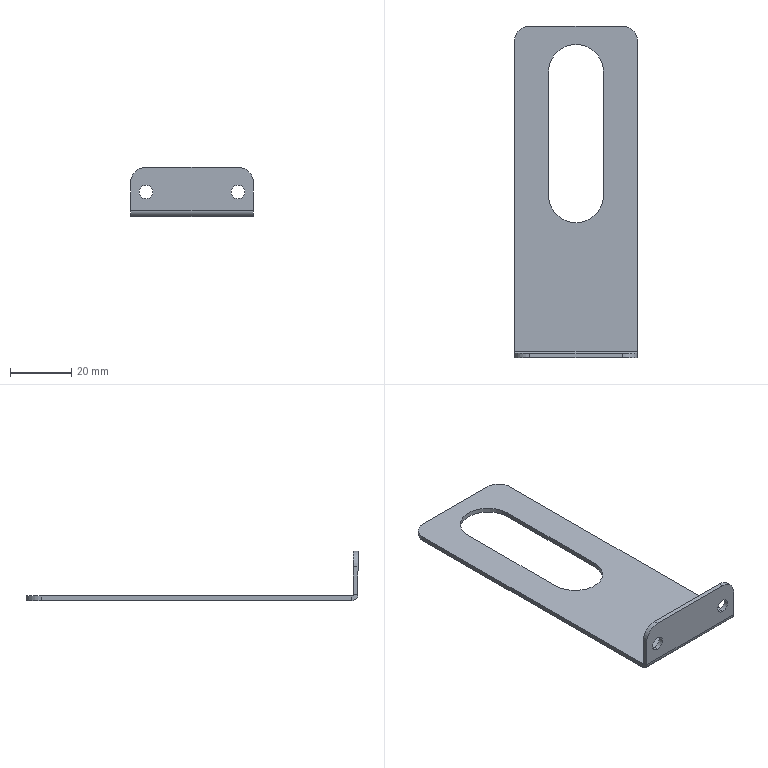Part | SolidWorks | features ICE 2, EdgeFlange 1, Fillet 1, FlatPattern 1, SMBaseFlange 1, SheetMetal 1 | 1 solid | 26 faces | box 40 x 108 x 16 mm | volume 5776 mm3 | plane 14 | cylinder 12 | commonest cylinder face diameters 4.5 x4 10 x4 18 x2 1 x1 4 x1
STEP:
#1=CARTESIAN_POINT('',(-15.,-54.,4.25));
#2=VERTEX_POINT('',#1);
#3=CARTESIAN_POINT('',(-15.,-54.,8.75));
#4=VERTEX_POINT('',#3);
#5=CARTESIAN_POINT('',(-15.,-54.,6.5));
#6=DIRECTION('',(0.,1.,0.));
#7=DIRECTION('',(0.,0.,1.));
#8=AXIS2_PLACEMENT_3D('',#5,#6,#7);
#9=CIRCLE('',#8,2.25);
#10=EDGE_CURVE('',#2,#4,#9,.T.);
#11=ORIENTED_EDGE('',*,*,#10,.F.);
#12=CARTESIAN_POINT('',(-15.,-52.5,4.25));
#13=VERTEX_POINT('',#12);
#14=CARTESIAN_POINT('',(-15.,-62.5,4.25));
#15=DIRECTION('',(0.,1.,0.));
#16=VECTOR('',#15,1000.);
#17=LINE('',#14,#16);
#18=EDGE_CURVE('',#2,#13,#17,.T.);
#19=ORIENTED_EDGE('',*,*,#18,.T.);
#20=CARTESIAN_POINT('',(-15.,-52.5,8.75));
#21=VERTEX_POINT('',#20);
#22=CARTESIAN_POINT('',(-15.,-52.5,6.5));
#23=DIRECTION('',(0.,1.,0.));
#24=DIRECTION('',(0.,0.,1.));
#25=AXIS2_PLACEMENT_3D('',#22,#23,#24);
#26=CIRCLE('',#25,2.25);
#27=EDGE_CURVE('',#13,#21,#26,.T.);
#28=ORIENTED_EDGE('',*,*,#27,.T.);
#29=CARTESIAN_POINT('',(-15.,-62.5,8.75));
#30=DIRECTION('',(0.,1.,0.));
#31=VECTOR('',#30,1000.);
#32=LINE('',#29,#31);
#33=EDGE_CURVE('',#4,#21,#32,.T.);
#34=ORIENTED_EDGE('',*,*,#33,.F.);
#35=EDGE_LOOP('',(#11,#19,#28,#34));
#36=FACE_OUTER_BOUND('',#35,.T.);
#37=CARTESIAN_POINT('',(-15.,-62.5,6.5));
#38=DIRECTION('',(0.,1.,0.));
#39=DIRECTION('',(0.,0.,1.));
#40=AXIS2_PLACEMENT_3D('',#37,#38,#39);
#41=CYLINDRICAL_SURFACE('',#40,2.25);
#42=ADVANCED_FACE('',(#36),#41,.F.);
#43=CARTESIAN_POINT('',(15.,-54.,4.25));
#44=VERTEX_POINT('',#43);
#45=CARTESIAN_POINT('',(15.,-54.,8.75));
#46=VERTEX_POINT('',#45);
#47=CARTESIAN_POINT('',(15.,-54.,6.5));
#48=DIRECTION('',(0.,1.,0.));
#49=DIRECTION('',(0.,0.,1.));
#50=AXIS2_PLACEMENT_3D('',#47,#48,#49);
#51=CIRCLE('',#50,2.25);
#52=EDGE_CURVE('',#44,#46,#51,.T.);
#53=ORIENTED_EDGE('',*,*,#52,.F.);
#54=CARTESIAN_POINT('',(15.,-52.5,4.25));
#55=VERTEX_POINT('',#54);
#56=CARTESIAN_POINT('',(15.,-62.5,4.25));
#57=DIRECTION('',(0.,1.,0.));
#58=VECTOR('',#57,1000.);
#59=LINE('',#56,#58);
#60=EDGE_CURVE('',#44,#55,#59,.T.);
#61=ORIENTED_EDGE('',*,*,#60,.T.);
#62=CARTESIAN_POINT('',(15.,-52.5,8.75));
#63=VERTEX_POINT('',#62);
#64=CARTESIAN_POINT('',(15.,-52.5,6.5));
#65=DIRECTION('',(0.,1.,0.));
#66=DIRECTION('',(0.,0.,-1.));
#67=AXIS2_PLACEMENT_3D('',#64,#65,#66);
#68=CIRCLE('',#67,2.25);
#69=EDGE_CURVE('',#55,#63,#68,.T.);
#70=ORIENTED_EDGE('',*,*,#69,.T.);
#71=CARTESIAN_POINT('',(15.,-62.5,8.75));
#72=DIRECTION('',(0.,1.,0.));
#73=VECTOR('',#72,1000.);
#74=LINE('',#71,#73);
#75=EDGE_CURVE('',#46,#63,#74,.T.);
#76=ORIENTED_EDGE('',*,*,#75,.F.);
#77=EDGE_LOOP('',(#53,#61,#70,#76));
#78=FACE_OUTER_BOUND('',#77,.T.);
#79=CARTESIAN_POINT('',(15.,-62.5,6.5));
#80=DIRECTION('',(0.,1.,0.));
#81=DIRECTION('',(0.,0.,1.));
#82=AXIS2_PLACEMENT_3D('',#79,#80,#81);
#83=CYLINDRICAL_SURFACE('',#82,2.25);
#84=ADVANCED_FACE('',(#78),#83,.F.);
#85=CARTESIAN_POINT('',(20.,-52.,-1.5));
#86=VERTEX_POINT('',#85);
#87=CARTESIAN_POINT('',(20.,49.,-1.5));
#88=VERTEX_POINT('',#87);
#89=CARTESIAN_POINT('',(20.,-54.,-1.5));
#90=DIRECTION('',(0.,1.,0.));
#91=VECTOR('',#90,1000.);
#92=LINE('',#89,#91);
#93=EDGE_CURVE('',#86,#88,#92,.T.);
#94=ORIENTED_EDGE('',*,*,#93,.T.);
#95=CARTESIAN_POINT('',(20.,49.,0.));
#96=VERTEX_POINT('',#95);
#97=CARTESIAN_POINT('',(20.,49.,-1.5));
#98=DIRECTION('',(0.,0.,1.));
#99=VECTOR('',#98,1000.);
#100=LINE('',#97,#99);
#101=EDGE_CURVE('',#88,#96,#100,.T.);
#102=ORIENTED_EDGE('',*,*,#101,.T.);
#103=CARTESIAN_POINT('',(20.,-52.,0.));
#104=VERTEX_POINT('',#103);
#105=CARTESIAN_POINT('',(20.,-54.,0.));
#106=DIRECTION('',(0.,1.,0.));
#107=VECTOR('',#106,1000.);
#108=LINE('',#105,#107);
#109=EDGE_CURVE('',#104,#96,#108,.T.);
#110=ORIENTED_EDGE('',*,*,#109,.F.);
#111=CARTESIAN_POINT('',(20.,-52.,0.));
#112=DIRECTION('',(0.,0.,-1.));
#113=VECTOR('',#112,1000.);
#114=LINE('',#111,#113);
#115=EDGE_CURVE('',#104,#86,#114,.T.);
#116=ORIENTED_EDGE('',*,*,#115,.T.);
#117=EDGE_LOOP('',(#94,#102,#110,#116));
#118=FACE_OUTER_BOUND('',#117,.T.);
#119=CARTESIAN_POINT('',(20.,-54.,-1.5));
#120=DIRECTION('',(1.,0.,0.));
#121=DIRECTION('',(0.,0.,-1.));
#122=AXIS2_PLACEMENT_3D('',#119,#120,#121);
#123=PLANE('',#122);
#124=ADVANCED_FACE('',(#118),#123,.T.);
#125=CARTESIAN_POINT('',(-9.,-1.,-1.5));
#126=VERTEX_POINT('',#125);
#127=CARTESIAN_POINT('',(9.,-1.,-1.5));
#128=VERTEX_POINT('',#127);
#129=CARTESIAN_POINT('',(0.,-1.,-1.5));
#130=DIRECTION('',(0.,0.,1.));
#131=DIRECTION('',(1.,0.,0.));
#132=AXIS2_PLACEMENT_3D('',#129,#130,#131);
#133=CIRCLE('',#132,9.);
#134=EDGE_CURVE('',#126,#128,#133,.T.);
#135=ORIENTED_EDGE('',*,*,#134,.T.);
#136=CARTESIAN_POINT('',(9.,39.,-1.5));
#137=VERTEX_POINT('',#136);
#138=CARTESIAN_POINT('',(9.,-1.,-1.5));
#139=DIRECTION('',(0.,1.,0.));
#140=VECTOR('',#139,1000.);
#141=LINE('',#138,#140);
#142=EDGE_CURVE('',#128,#137,#141,.T.);
#143=ORIENTED_EDGE('',*,*,#142,.T.);
#144=CARTESIAN_POINT('',(-9.,39.,-1.5));
#145=VERTEX_POINT('',#144);
#146=CARTESIAN_POINT('',(0.,39.,-1.5));
#147=DIRECTION('',(0.,0.,1.));
#148=DIRECTION('',(1.,0.,0.));
#149=AXIS2_PLACEMENT_3D('',#146,#147,#148);
#150=CIRCLE('',#149,9.);
#151=EDGE_CURVE('',#137,#145,#150,.T.);
#152=ORIENTED_EDGE('',*,*,#151,.T.);
#153=CARTESIAN_POINT('',(-9.,-1.,-1.5));
#154=DIRECTION('',(0.,-1.,0.));
#155=VECTOR('',#154,1000.);
#156=LINE('',#153,#155);
#157=EDGE_CURVE('',#145,#126,#156,.T.);
#158=ORIENTED_EDGE('',*,*,#157,.T.);
#159=EDGE_LOOP('',(#135,#143,#152,#158));
#160=FACE_BOUND('',#159,.T.);
#161=CARTESIAN_POINT('',(15.,54.,-1.5));
#162=VERTEX_POINT('',#161);
#163=CARTESIAN_POINT('',(-15.,54.,-1.5));
#164=VERTEX_POINT('',#163);
#165=CARTESIAN_POINT('',(-20.,54.,-1.5));
#166=DIRECTION('',(-1.,0.,0.));
#167=VECTOR('',#166,1000.);
#168=LINE('',#165,#167);
#169=EDGE_CURVE('',#162,#164,#168,.T.);
#170=ORIENTED_EDGE('',*,*,#169,.F.);
#171=CARTESIAN_POINT('',(15.,49.,-1.5));
#172=DIRECTION('',(0.,0.,-1.));
#173=DIRECTION('',(-1.,0.,0.));
#174=AXIS2_PLACEMENT_3D('',#171,#172,#173);
#175=CIRCLE('',#174,5.);
#176=EDGE_CURVE('',#162,#88,#175,.T.);
#177=ORIENTED_EDGE('',*,*,#176,.T.);
#178=ORIENTED_EDGE('',*,*,#93,.F.);
#179=CARTESIAN_POINT('',(-20.,-52.,-1.5));
#180=VERTEX_POINT('',#179);
#181=CARTESIAN_POINT('',(20.,-52.,-1.5));
#182=DIRECTION('',(-1.,0.,0.));
#183=VECTOR('',#182,1000.);
#184=LINE('',#181,#183);
#185=EDGE_CURVE('',#86,#180,#184,.T.);
#186=ORIENTED_EDGE('',*,*,#185,.T.);
#187=CARTESIAN_POINT('',(-20.,49.,-1.5));
#188=VERTEX_POINT('',#187);
#189=CARTESIAN_POINT('',(-20.,-54.,-1.5));
#190=DIRECTION('',(0.,-1.,0.));
#191=VECTOR('',#190,1000.);
#192=LINE('',#189,#191);
#193=EDGE_CURVE('',#188,#180,#192,.T.);
#194=ORIENTED_EDGE('',*,*,#193,.F.);
#195=CARTESIAN_POINT('',(-15.,49.,-1.5));
#196=DIRECTION('',(0.,0.,-1.));
#197=DIRECTION('',(-1.,0.,0.));
#198=AXIS2_PLACEMENT_3D('',#195,#196,#197);
#199=CIRCLE('',#198,5.);
#200=EDGE_CURVE('',#188,#164,#199,.T.);
#201=ORIENTED_EDGE('',*,*,#200,.T.);
#202=EDGE_LOOP('',(#170,#177,#178,#186,#194,#201));
#203=FACE_OUTER_BOUND('',#202,.T.);
#204=CARTESIAN_POINT('',(0.,0.,-1.5));
#205=DIRECTION('',(0.,0.,-1.));
#206=DIRECTION('',(-1.,0.,0.));
#207=AXIS2_PLACEMENT_3D('',#204,#205,#206);
#208=PLANE('',#207);
#209=ADVANCED_FACE('',(#160,#203),#208,.T.);
#210=CARTESIAN_POINT('',(9.,-1.,0.));
#211=VERTEX_POINT('',#210);
#212=CARTESIAN_POINT('',(9.,39.,0.));
#213=VERTEX_POINT('',#212);
#214=CARTESIAN_POINT('',(9.,-1.,0.));
#215=DIRECTION('',(0.,1.,0.));
#216=VECTOR('',#215,1000.);
#217=LINE('',#214,#216);
#218=EDGE_CURVE('',#211,#213,#217,.T.);
#219=ORIENTED_EDGE('',*,*,#218,.F.);
#220=CARTESIAN_POINT('',(-9.,-1.,0.));
#221=VERTEX_POINT('',#220);
#222=CARTESIAN_POINT('',(0.,-1.,0.));
#223=DIRECTION('',(0.,0.,1.));
#224=DIRECTION('',(1.,0.,0.));
#225=AXIS2_PLACEMENT_3D('',#222,#223,#224);
#226=CIRCLE('',#225,9.);
#227=EDGE_CURVE('',#221,#211,#226,.T.);
#228=ORIENTED_EDGE('',*,*,#227,.F.);
#229=CARTESIAN_POINT('',(-9.,39.,0.));
#230=VERTEX_POINT('',#229);
#231=CARTESIAN_POINT('',(-9.,-1.,0.));
#232=DIRECTION('',(0.,-1.,0.));
#233=VECTOR('',#232,1000.);
#234=LINE('',#231,#233);
#235=EDGE_CURVE('',#230,#221,#234,.T.);
#236=ORIENTED_EDGE('',*,*,#235,.F.);
#237=CARTESIAN_POINT('',(0.,39.,0.));
#238=DIRECTION('',(0.,0.,1.));
#239=DIRECTION('',(1.,0.,0.));
#240=AXIS2_PLACEMENT_3D('',#237,#238,#239);
#241=CIRCLE('',#240,9.);
#242=EDGE_CURVE('',#213,#230,#241,.T.);
#243=ORIENTED_EDGE('',*,*,#242,.F.);
#244=EDGE_LOOP('',(#219,#228,#236,#243));
#245=FACE_BOUND('',#244,.T.);
#246=ORIENTED_EDGE('',*,*,#109,.T.);
#247=CARTESIAN_POINT('',(15.,54.,0.));
#248=VERTEX_POINT('',#247);
#249=CARTESIAN_POINT('',(15.,49.,0.));
#250=DIRECTION('',(0.,0.,1.));
#251=DIRECTION('',(-1.,0.,0.));
#252=AXIS2_PLACEMENT_3D('',#249,#250,#251);
#253=CIRCLE('',#252,5.);
#254=EDGE_CURVE('',#96,#248,#253,.T.);
#255=ORIENTED_EDGE('',*,*,#254,.T.);
#256=CARTESIAN_POINT('',(-15.,54.,0.));
#257=VERTEX_POINT('',#256);
#258=CARTESIAN_POINT('',(-20.,54.,0.));
#259=DIRECTION('',(-1.,0.,0.));
#260=VECTOR('',#259,1000.);
#261=LINE('',#258,#260);
#262=EDGE_CURVE('',#248,#257,#261,.T.);
#263=ORIENTED_EDGE('',*,*,#262,.T.);
#264=CARTESIAN_POINT('',(-20.,49.,0.));
#265=VERTEX_POINT('',#264);
#266=CARTESIAN_POINT('',(-15.,49.,0.));
#267=DIRECTION('',(0.,0.,1.));
#268=DIRECTION('',(-1.,0.,0.));
#269=AXIS2_PLACEMENT_3D('',#266,#267,#268);
#270=CIRCLE('',#269,5.);
#271=EDGE_CURVE('',#257,#265,#270,.T.);
#272=ORIENTED_EDGE('',*,*,#271,.T.);
#273=CARTESIAN_POINT('',(-20.,-52.,0.));
#274=VERTEX_POINT('',#273);
#275=CARTESIAN_POINT('',(-20.,-54.,0.));
#276=DIRECTION('',(0.,-1.,0.));
#277=VECTOR('',#276,1000.);
#278=LINE('',#275,#277);
#279=EDGE_CURVE('',#265,#274,#278,.T.);
#280=ORIENTED_EDGE('',*,*,#279,.T.);
#281=CARTESIAN_POINT('',(20.,-52.,0.));
#282=DIRECTION('',(-1.,0.,0.));
#283=VECTOR('',#282,1000.);
#284=LINE('',#281,#283);
#285=EDGE_CURVE('',#104,#274,#284,.T.);
#286=ORIENTED_EDGE('',*,*,#285,.F.);
#287=EDGE_LOOP('',(#246,#255,#263,#272,#280,#286));
#288=FACE_OUTER_BOUND('',#287,.T.);
#289=CARTESIAN_POINT('',(0.,0.,0.));
#290=DIRECTION('',(0.,0.,-1.));
#291=DIRECTION('',(-1.,0.,0.));
#292=AXIS2_PLACEMENT_3D('',#289,#290,#291);
#293=PLANE('',#292);
#294=ADVANCED_FACE('',(#245,#288),#293,.F.);
#295=ORIENTED_EDGE('',*,*,#279,.F.);
#296=CARTESIAN_POINT('',(-20.,49.,-1.5));
#297=DIRECTION('',(0.,0.,-1.));
#298=VECTOR('',#297,1000.);
#299=LINE('',#296,#298);
#300=EDGE_CURVE('',#265,#188,#299,.T.);
#301=ORIENTED_EDGE('',*,*,#300,.T.);
#302=ORIENTED_EDGE('',*,*,#193,.T.);
#303=CARTESIAN_POINT('',(-20.,-52.,0.));
#304=DIRECTION('',(0.,0.,-1.));
#305=VECTOR('',#304,1000.);
#306=LINE('',#303,#305);
#307=EDGE_CURVE('',#274,#180,#306,.T.);
#308=ORIENTED_EDGE('',*,*,#307,.F.);
#309=EDGE_LOOP('',(#295,#301,#302,#308));
#310=FACE_OUTER_BOUND('',#309,.T.);
#311=CARTESIAN_POINT('',(-20.,-54.,-1.5));
#312=DIRECTION('',(-1.,0.,0.));
#313=DIRECTION('',(0.,0.,1.));
#314=AXIS2_PLACEMENT_3D('',#311,#312,#313);
#315=PLANE('',#314);
#316=ADVANCED_FACE('',(#310),#315,.T.);
#317=ORIENTED_EDGE('',*,*,#262,.F.);
#318=CARTESIAN_POINT('',(15.,54.,-1.5));
#319=DIRECTION('',(0.,0.,-1.));
#320=VECTOR('',#319,1000.);
#321=LINE('',#318,#320);
#322=EDGE_CURVE('',#248,#162,#321,.T.);
#323=ORIENTED_EDGE('',*,*,#322,.T.);
#324=ORIENTED_EDGE('',*,*,#169,.T.);
#325=CARTESIAN_POINT('',(-15.,54.,-1.5));
#326=DIRECTION('',(0.,0.,1.));
#327=VECTOR('',#326,1000.);
#328=LINE('',#325,#327);
#329=EDGE_CURVE('',#164,#257,#328,.T.);
#330=ORIENTED_EDGE('',*,*,#329,.T.);
#331=EDGE_LOOP('',(#317,#323,#324,#330));
#332=FACE_OUTER_BOUND('',#331,.T.);
#333=CARTESIAN_POINT('',(-20.,54.,-1.5));
#334=DIRECTION('',(0.,1.,0.));
#335=DIRECTION('',(0.,0.,1.));
#336=AXIS2_PLACEMENT_3D('',#333,#334,#335);
#337=PLANE('',#336);
#338=ADVANCED_FACE('',(#332),#337,.T.);
#339=CARTESIAN_POINT('',(-20.,-52.5,0.5));
#340=VERTEX_POINT('',#339);
#341=CARTESIAN_POINT('',(-20.,-54.,0.5));
#342=VERTEX_POINT('',#341);
#343=CARTESIAN_POINT('',(-20.,-54.,0.5));
#344=DIRECTION('',(0.,-1.,0.));
#345=VECTOR('',#344,1000.);
#346=LINE('',#343,#345);
#347=EDGE_CURVE('',#340,#342,#346,.T.);
#348=ORIENTED_EDGE('',*,*,#347,.F.);
#349=CARTESIAN_POINT('',(-20.,-52.,0.5));
#350=DIRECTION('',(-1.,0.,0.));
#351=DIRECTION('',(0.,0.,-1.));
#352=AXIS2_PLACEMENT_3D('',#349,#350,#351);
#353=CIRCLE('',#352,0.5);
#354=EDGE_CURVE('',#274,#340,#353,.T.);
#355=ORIENTED_EDGE('',*,*,#354,.F.);
#356=ORIENTED_EDGE('',*,*,#307,.T.);
#357=CARTESIAN_POINT('',(-20.,-52.,0.5));
#358=DIRECTION('',(-1.,0.,0.));
#359=DIRECTION('',(0.,0.,-1.));
#360=AXIS2_PLACEMENT_3D('',#357,#358,#359);
#361=CIRCLE('',#360,2.);
#362=EDGE_CURVE('',#180,#342,#361,.T.);
#363=ORIENTED_EDGE('',*,*,#362,.T.);
#364=EDGE_LOOP('',(#348,#355,#356,#363));
#365=FACE_OUTER_BOUND('',#364,.T.);
#366=CARTESIAN_POINT('',(-20.,-52.,0.5));
#367=DIRECTION('',(-1.,0.,0.));
#368=DIRECTION('',(0.,0.,1.));
#369=AXIS2_PLACEMENT_3D('',#366,#367,#368);
#370=PLANE('',#369);
#371=ADVANCED_FACE('',(#365),#370,.T.);
#372=CARTESIAN_POINT('',(20.,-52.5,0.5));
#373=VERTEX_POINT('',#372);
#374=CARTESIAN_POINT('',(20.,-52.,0.5));
#375=DIRECTION('',(1.,0.,0.));
#376=DIRECTION('',(0.,0.,-1.));
#377=AXIS2_PLACEMENT_3D('',#374,#375,#376);
#378=CIRCLE('',#377,0.5);
#379=EDGE_CURVE('',#373,#104,#378,.T.);
#380=ORIENTED_EDGE('',*,*,#379,.F.);
#381=CARTESIAN_POINT('',(20.,-54.,0.5));
#382=VERTEX_POINT('',#381);
#383=CARTESIAN_POINT('',(20.,-52.5,0.5));
#384=DIRECTION('',(0.,-1.,0.));
#385=VECTOR('',#384,1000.);
#386=LINE('',#383,#385);
#387=EDGE_CURVE('',#373,#382,#386,.T.);
#388=ORIENTED_EDGE('',*,*,#387,.T.);
#389=CARTESIAN_POINT('',(20.,-52.,0.5));
#390=DIRECTION('',(1.,0.,0.));
#391=DIRECTION('',(0.,0.,-1.));
#392=AXIS2_PLACEMENT_3D('',#389,#390,#391);
#393=CIRCLE('',#392,2.);
#394=EDGE_CURVE('',#382,#86,#393,.T.);
#395=ORIENTED_EDGE('',*,*,#394,.T.);
#396=ORIENTED_EDGE('',*,*,#115,.F.);
#397=EDGE_LOOP('',(#380,#388,#395,#396));
#398=FACE_OUTER_BOUND('',#397,.T.);
#399=CARTESIAN_POINT('',(20.,-52.,0.5));
#400=DIRECTION('',(-1.,0.,0.));
#401=DIRECTION('',(0.,0.,1.));
#402=AXIS2_PLACEMENT_3D('',#399,#400,#401);
#403=PLANE('',#402);
#404=ADVANCED_FACE('',(#398),#403,.F.);
#405=ORIENTED_EDGE('',*,*,#185,.F.);
#406=ORIENTED_EDGE('',*,*,#394,.F.);
#407=CARTESIAN_POINT('',(-20.,-54.,0.5));
#408=DIRECTION('',(-1.,0.,0.));
#409=VECTOR('',#408,1000.);
#410=LINE('',#407,#409);
#411=EDGE_CURVE('',#382,#342,#410,.T.);
#412=ORIENTED_EDGE('',*,*,#411,.T.);
#413=ORIENTED_EDGE('',*,*,#362,.F.);
#414=EDGE_LOOP('',(#405,#406,#412,#413));
#415=FACE_OUTER_BOUND('',#414,.T.);
#416=CARTESIAN_POINT('',(20.,-52.,0.5));
#417=DIRECTION('',(1.,0.,0.));
#418=DIRECTION('',(0.,-1.,0.));
#419=AXIS2_PLACEMENT_3D('',#416,#417,#418);
#420=CYLINDRICAL_SURFACE('',#419,2.);
#421=ADVANCED_FACE('',(#415),#420,.T.);
#422=ORIENTED_EDGE('',*,*,#285,.T.);
#423=ORIENTED_EDGE('',*,*,#354,.T.);
#424=CARTESIAN_POINT('',(-20.,-52.5,0.5));
#425=DIRECTION('',(1.,0.,0.));
#426=VECTOR('',#425,1000.);
#427=LINE('',#424,#426);
#428=EDGE_CURVE('',#340,#373,#427,.T.);
#429=ORIENTED_EDGE('',*,*,#428,.T.);
#430=ORIENTED_EDGE('',*,*,#379,.T.);
#431=EDGE_LOOP('',(#422,#423,#429,#430));
#432=FACE_OUTER_BOUND('',#431,.T.);
#433=CARTESIAN_POINT('',(20.,-52.,0.5));
#434=DIRECTION('',(1.,0.,0.));
#435=DIRECTION('',(0.,-1.,0.));
#436=AXIS2_PLACEMENT_3D('',#433,#434,#435);
#437=CYLINDRICAL_SURFACE('',#436,0.5);
#438=ADVANCED_FACE('',(#432),#437,.F.);
#439=CARTESIAN_POINT('',(-20.,-54.,9.5));
#440=VERTEX_POINT('',#439);
#441=CARTESIAN_POINT('',(-20.,-54.,0.));
#442=DIRECTION('',(0.,0.,-1.));
#443=VECTOR('',#442,1000.);
#444=LINE('',#441,#443);
#445=EDGE_CURVE('',#440,#342,#444,.T.);
#446=ORIENTED_EDGE('',*,*,#445,.F.);
#447=CARTESIAN_POINT('',(-20.,-52.5,9.5));
#448=VERTEX_POINT('',#447);
#449=CARTESIAN_POINT('',(-20.,-54.,9.5));
#450=DIRECTION('',(0.,1.,0.));
#451=VECTOR('',#450,1000.);
#452=LINE('',#449,#451);
#453=EDGE_CURVE('',#440,#448,#452,.T.);
#454=ORIENTED_EDGE('',*,*,#453,.T.);
#455=CARTESIAN_POINT('',(-20.,-52.5,0.));
#456=DIRECTION('',(0.,0.,-1.));
#457=VECTOR('',#456,1000.);
#458=LINE('',#455,#457);
#459=EDGE_CURVE('',#448,#340,#458,.T.);
#460=ORIENTED_EDGE('',*,*,#459,.T.);
#461=ORIENTED_EDGE('',*,*,#347,.T.);
#462=EDGE_LOOP('',(#446,#454,#460,#461));
#463=FACE_OUTER_BOUND('',#462,.T.);
#464=CARTESIAN_POINT('',(-20.,-54.,0.));
#465=DIRECTION('',(1.,0.,0.));
#466=DIRECTION('',(0.,0.,-1.));
#467=AXIS2_PLACEMENT_3D('',#464,#465,#466);
#468=PLANE('',#467);
#469=ADVANCED_FACE('',(#463),#468,.F.);
#470=CARTESIAN_POINT('',(20.,-52.5,9.5));
#471=VERTEX_POINT('',#470);
#472=CARTESIAN_POINT('',(20.,-52.5,14.5));
#473=DIRECTION('',(0.,0.,1.));
#474=VECTOR('',#473,1000.);
#475=LINE('',#472,#474);
#476=EDGE_CURVE('',#373,#471,#475,.T.);
#477=ORIENTED_EDGE('',*,*,#476,.T.);
#478=CARTESIAN_POINT('',(20.,-54.,9.5));
#479=VERTEX_POINT('',#478);
#480=CARTESIAN_POINT('',(20.,-54.,9.5));
#481=DIRECTION('',(0.,-1.,0.));
#482=VECTOR('',#481,1000.);
#483=LINE('',#480,#482);
#484=EDGE_CURVE('',#471,#479,#483,.T.);
#485=ORIENTED_EDGE('',*,*,#484,.T.);
#486=CARTESIAN_POINT('',(20.,-54.,0.));
#487=DIRECTION('',(0.,0.,1.));
#488=VECTOR('',#487,1000.);
#489=LINE('',#486,#488);
#490=EDGE_CURVE('',#382,#479,#489,.T.);
#491=ORIENTED_EDGE('',*,*,#490,.F.);
#492=ORIENTED_EDGE('',*,*,#387,.F.);
#493=EDGE_LOOP('',(#477,#485,#491,#492));
#494=FACE_OUTER_BOUND('',#493,.T.);
#495=CARTESIAN_POINT('',(20.,-54.,14.5));
#496=DIRECTION('',(-1.,0.,0.));
#497=DIRECTION('',(0.,0.,1.));
#498=AXIS2_PLACEMENT_3D('',#495,#496,#497);
#499=PLANE('',#498);
#500=ADVANCED_FACE('',(#494),#499,.F.);
#501=CARTESIAN_POINT('',(-15.,-54.,6.5));
#502=DIRECTION('',(0.,1.,0.));
#503=DIRECTION('',(0.,0.,1.));
#504=AXIS2_PLACEMENT_3D('',#501,#502,#503);
#505=CIRCLE('',#504,2.25);
#506=EDGE_CURVE('',#4,#2,#505,.T.);
#507=ORIENTED_EDGE('',*,*,#506,.T.);
#508=ORIENTED_EDGE('',*,*,#10,.T.);
#509=EDGE_LOOP('',(#507,#508));
#510=FACE_BOUND('',#509,.T.);
#511=CARTESIAN_POINT('',(15.,-54.,6.5));
#512=DIRECTION('',(0.,1.,0.));
#513=DIRECTION('',(0.,0.,1.));
#514=AXIS2_PLACEMENT_3D('',#511,#512,#513);
#515=CIRCLE('',#514,2.25);
#516=EDGE_CURVE('',#46,#44,#515,.T.);
#517=ORIENTED_EDGE('',*,*,#516,.T.);
#518=ORIENTED_EDGE('',*,*,#52,.T.);
#519=EDGE_LOOP('',(#517,#518));
#520=FACE_BOUND('',#519,.T.);
#521=ORIENTED_EDGE('',*,*,#490,.T.);
#522=CARTESIAN_POINT('',(15.,-54.,14.5));
#523=VERTEX_POINT('',#522);
#524=CARTESIAN_POINT('',(15.,-54.,9.5));
#525=DIRECTION('',(0.,-1.,0.));
#526=DIRECTION('',(0.,0.,1.));
#527=AXIS2_PLACEMENT_3D('',#524,#525,#526);
#528=CIRCLE('',#527,5.);
#529=EDGE_CURVE('',#479,#523,#528,.T.);
#530=ORIENTED_EDGE('',*,*,#529,.T.);
#531=CARTESIAN_POINT('',(-15.,-54.,14.5));
#532=VERTEX_POINT('',#531);
#533=CARTESIAN_POINT('',(0.,-54.,14.5));
#534=DIRECTION('',(-1.,0.,0.));
#535=VECTOR('',#534,1000.);
#536=LINE('',#533,#535);
#537=EDGE_CURVE('',#523,#532,#536,.T.);
#538=ORIENTED_EDGE('',*,*,#537,.T.);
#539=CARTESIAN_POINT('',(-15.,-54.,9.5));
#540=DIRECTION('',(0.,-1.,0.));
#541=DIRECTION('',(0.,0.,1.));
#542=AXIS2_PLACEMENT_3D('',#539,#540,#541);
#543=CIRCLE('',#542,5.);
#544=EDGE_CURVE('',#532,#440,#543,.T.);
#545=ORIENTED_EDGE('',*,*,#544,.T.);
#546=ORIENTED_EDGE('',*,*,#445,.T.);
#547=ORIENTED_EDGE('',*,*,#411,.F.);
#548=EDGE_LOOP('',(#521,#530,#538,#545,#546,#547));
#549=FACE_OUTER_BOUND('',#548,.T.);
#550=CARTESIAN_POINT('',(0.,-54.,0.));
#551=DIRECTION('',(0.,1.,0.));
#552=DIRECTION('',(0.,0.,1.));
#553=AXIS2_PLACEMENT_3D('',#550,#551,#552);
#554=PLANE('',#553);
#555=ADVANCED_FACE('',(#510,#520,#549),#554,.F.);
#556=CARTESIAN_POINT('',(-15.,-52.5,6.5));
#557=DIRECTION('',(0.,1.,0.));
#558=DIRECTION('',(0.,0.,1.));
#559=AXIS2_PLACEMENT_3D('',#556,#557,#558);
#560=CIRCLE('',#559,2.25);
#561=EDGE_CURVE('',#21,#13,#560,.T.);
#562=ORIENTED_EDGE('',*,*,#561,.F.);
#563=ORIENTED_EDGE('',*,*,#27,.F.);
#564=EDGE_LOOP('',(#562,#563));
#565=FACE_BOUND('',#564,.T.);
#566=CARTESIAN_POINT('',(15.,-52.5,6.5));
#567=DIRECTION('',(0.,1.,0.));
#568=DIRECTION('',(0.,0.,-1.));
#569=AXIS2_PLACEMENT_3D('',#566,#567,#568);
#570=CIRCLE('',#569,2.25);
#571=EDGE_CURVE('',#63,#55,#570,.T.);
#572=ORIENTED_EDGE('',*,*,#571,.F.);
#573=ORIENTED_EDGE('',*,*,#69,.F.);
#574=EDGE_LOOP('',(#572,#573));
#575=FACE_BOUND('',#574,.T.);
#576=CARTESIAN_POINT('',(15.,-52.5,14.5));
#577=VERTEX_POINT('',#576);
#578=CARTESIAN_POINT('',(-15.,-52.5,14.5));
#579=VERTEX_POINT('',#578);
#580=CARTESIAN_POINT('',(-20.,-52.5,14.5));
#581=DIRECTION('',(-1.,0.,0.));
#582=VECTOR('',#581,1000.);
#583=LINE('',#580,#582);
#584=EDGE_CURVE('',#577,#579,#583,.T.);
#585=ORIENTED_EDGE('',*,*,#584,.F.);
#586=CARTESIAN_POINT('',(15.,-52.5,9.5));
#587=DIRECTION('',(0.,1.,0.));
#588=DIRECTION('',(0.,0.,1.));
#589=AXIS2_PLACEMENT_3D('',#586,#587,#588);
#590=CIRCLE('',#589,5.);
#591=EDGE_CURVE('',#577,#471,#590,.T.);
#592=ORIENTED_EDGE('',*,*,#591,.T.);
#593=ORIENTED_EDGE('',*,*,#476,.F.);
#594=ORIENTED_EDGE('',*,*,#428,.F.);
#595=ORIENTED_EDGE('',*,*,#459,.F.);
#596=CARTESIAN_POINT('',(-15.,-52.5,9.5));
#597=DIRECTION('',(0.,1.,0.));
#598=DIRECTION('',(0.,0.,1.));
#599=AXIS2_PLACEMENT_3D('',#596,#597,#598);
#600=CIRCLE('',#599,5.);
#601=EDGE_CURVE('',#448,#579,#600,.T.);
#602=ORIENTED_EDGE('',*,*,#601,.T.);
#603=EDGE_LOOP('',(#585,#592,#593,#594,#595,#602));
#604=FACE_OUTER_BOUND('',#603,.T.);
#605=CARTESIAN_POINT('',(0.,-52.5,0.));
#606=DIRECTION('',(0.,1.,0.));
#607=DIRECTION('',(0.,0.,1.));
#608=AXIS2_PLACEMENT_3D('',#605,#606,#607);
#609=PLANE('',#608);
#610=ADVANCED_FACE('',(#565,#575,#604),#609,.T.);
#611=ORIENTED_EDGE('',*,*,#537,.F.);
#612=CARTESIAN_POINT('',(15.,-54.,14.5));
#613=DIRECTION('',(0.,1.,0.));
#614=VECTOR('',#613,1000.);
#615=LINE('',#612,#614);
#616=EDGE_CURVE('',#523,#577,#615,.T.);
#617=ORIENTED_EDGE('',*,*,#616,.T.);
#618=ORIENTED_EDGE('',*,*,#584,.T.);
#619=CARTESIAN_POINT('',(-15.,-54.,14.5));
#620=DIRECTION('',(0.,-1.,0.));
#621=VECTOR('',#620,1000.);
#622=LINE('',#619,#621);
#623=EDGE_CURVE('',#579,#532,#622,.T.);
#624=ORIENTED_EDGE('',*,*,#623,.T.);
#625=EDGE_LOOP('',(#611,#617,#618,#624));
#626=FACE_OUTER_BOUND('',#625,.T.);
#627=CARTESIAN_POINT('',(-20.,-54.,14.5));
#628=DIRECTION('',(0.,0.,-1.));
#629=DIRECTION('',(0.,1.,0.));
#630=AXIS2_PLACEMENT_3D('',#627,#628,#629);
#631=PLANE('',#630);
#632=ADVANCED_FACE('',(#626),#631,.F.);
#633=ORIENTED_EDGE('',*,*,#227,.T.);
#634=CARTESIAN_POINT('',(9.,-1.,-1.5));
#635=DIRECTION('',(0.,0.,1.));
#636=VECTOR('',#635,1000.);
#637=LINE('',#634,#636);
#638=EDGE_CURVE('',#128,#211,#637,.T.);
#639=ORIENTED_EDGE('',*,*,#638,.F.);
#640=ORIENTED_EDGE('',*,*,#134,.F.);
#641=CARTESIAN_POINT('',(-9.,-1.,-1.5));
#642=DIRECTION('',(0.,0.,1.));
#643=VECTOR('',#642,1000.);
#644=LINE('',#641,#643);
#645=EDGE_CURVE('',#126,#221,#644,.T.);
#646=ORIENTED_EDGE('',*,*,#645,.T.);
#647=EDGE_LOOP('',(#633,#639,#640,#646));
#648=FACE_OUTER_BOUND('',#647,.T.);
#649=CARTESIAN_POINT('',(0.,-1.,-1.5));
#650=DIRECTION('',(0.,0.,1.));
#651=DIRECTION('',(1.,0.,0.));
#652=AXIS2_PLACEMENT_3D('',#649,#650,#651);
#653=CYLINDRICAL_SURFACE('',#652,9.);
#654=ADVANCED_FACE('',(#648),#653,.F.);
#655=ORIENTED_EDGE('',*,*,#235,.T.);
#656=ORIENTED_EDGE('',*,*,#645,.F.);
#657=ORIENTED_EDGE('',*,*,#157,.F.);
#658=CARTESIAN_POINT('',(-9.,39.,-1.5));
#659=DIRECTION('',(0.,0.,1.));
#660=VECTOR('',#659,1000.);
#661=LINE('',#658,#660);
#662=EDGE_CURVE('',#145,#230,#661,.T.);
#663=ORIENTED_EDGE('',*,*,#662,.T.);
#664=EDGE_LOOP('',(#655,#656,#657,#663));
#665=FACE_OUTER_BOUND('',#664,.T.);
#666=CARTESIAN_POINT('',(-9.,-1.,-1.5));
#667=DIRECTION('',(-1.,0.,0.));
#668=DIRECTION('',(0.,-1.,0.));
#669=AXIS2_PLACEMENT_3D('',#666,#667,#668);
#670=PLANE('',#669);
#671=ADVANCED_FACE('',(#665),#670,.F.);
#672=ORIENTED_EDGE('',*,*,#242,.T.);
#673=ORIENTED_EDGE('',*,*,#662,.F.);
#674=ORIENTED_EDGE('',*,*,#151,.F.);
#675=CARTESIAN_POINT('',(9.,39.,-1.5));
#676=DIRECTION('',(0.,0.,1.));
#677=VECTOR('',#676,1000.);
#678=LINE('',#675,#677);
#679=EDGE_CURVE('',#137,#213,#678,.T.);
#680=ORIENTED_EDGE('',*,*,#679,.T.);
#681=EDGE_LOOP('',(#672,#673,#674,#680));
#682=FACE_OUTER_BOUND('',#681,.T.);
#683=CARTESIAN_POINT('',(0.,39.,-1.5));
#684=DIRECTION('',(0.,0.,1.));
#685=DIRECTION('',(1.,0.,0.));
#686=AXIS2_PLACEMENT_3D('',#683,#684,#685);
#687=CYLINDRICAL_SURFACE('',#686,9.);
#688=ADVANCED_FACE('',(#682),#687,.F.);
#689=ORIENTED_EDGE('',*,*,#218,.T.);
#690=ORIENTED_EDGE('',*,*,#679,.F.);
#691=ORIENTED_EDGE('',*,*,#142,.F.);
#692=ORIENTED_EDGE('',*,*,#638,.T.);
#693=EDGE_LOOP('',(#689,#690,#691,#692));
#694=FACE_OUTER_BOUND('',#693,.T.);
#695=CARTESIAN_POINT('',(9.,-1.,-1.5));
#696=DIRECTION('',(1.,0.,0.));
#697=DIRECTION('',(0.,1.,0.));
#698=AXIS2_PLACEMENT_3D('',#695,#696,#697);
#699=PLANE('',#698);
#700=ADVANCED_FACE('',(#694),#699,.F.);
#701=ORIENTED_EDGE('',*,*,#529,.F.);
#702=ORIENTED_EDGE('',*,*,#484,.F.);
#703=ORIENTED_EDGE('',*,*,#591,.F.);
#704=ORIENTED_EDGE('',*,*,#616,.F.);
#705=EDGE_LOOP('',(#701,#702,#703,#704));
#706=FACE_OUTER_BOUND('',#705,.T.);
#707=CARTESIAN_POINT('',(15.,-54.,9.5));
#708=DIRECTION('',(0.,1.,0.));
#709=DIRECTION('',(0.,0.,1.));
#710=AXIS2_PLACEMENT_3D('',#707,#708,#709);
#711=CYLINDRICAL_SURFACE('',#710,5.);
#712=ADVANCED_FACE('',(#706),#711,.T.);
#713=ORIENTED_EDGE('',*,*,#544,.F.);
#714=ORIENTED_EDGE('',*,*,#623,.F.);
#715=ORIENTED_EDGE('',*,*,#601,.F.);
#716=ORIENTED_EDGE('',*,*,#453,.F.);
#717=EDGE_LOOP('',(#713,#714,#715,#716));
#718=FACE_OUTER_BOUND('',#717,.T.);
#719=CARTESIAN_POINT('',(-15.,-54.,9.5));
#720=DIRECTION('',(0.,1.,0.));
#721=DIRECTION('',(0.,0.,1.));
#722=AXIS2_PLACEMENT_3D('',#719,#720,#721);
#723=CYLINDRICAL_SURFACE('',#722,5.);
#724=ADVANCED_FACE('',(#718),#723,.T.);
#725=ORIENTED_EDGE('',*,*,#176,.F.);
#726=ORIENTED_EDGE('',*,*,#322,.F.);
#727=ORIENTED_EDGE('',*,*,#254,.F.);
#728=ORIENTED_EDGE('',*,*,#101,.F.);
#729=EDGE_LOOP('',(#725,#726,#727,#728));
#730=FACE_OUTER_BOUND('',#729,.T.);
#731=CARTESIAN_POINT('',(15.,49.,-1.5));
#732=DIRECTION('',(0.,0.,1.));
#733=DIRECTION('',(1.,0.,0.));
#734=AXIS2_PLACEMENT_3D('',#731,#732,#733);
#735=CYLINDRICAL_SURFACE('',#734,5.);
#736=ADVANCED_FACE('',(#730),#735,.T.);
#737=ORIENTED_EDGE('',*,*,#200,.F.);
#738=ORIENTED_EDGE('',*,*,#300,.F.);
#739=ORIENTED_EDGE('',*,*,#271,.F.);
#740=ORIENTED_EDGE('',*,*,#329,.F.);
#741=EDGE_LOOP('',(#737,#738,#739,#740));
#742=FACE_OUTER_BOUND('',#741,.T.);
#743=CARTESIAN_POINT('',(-15.,49.,-1.5));
#744=DIRECTION('',(0.,0.,1.));
#745=DIRECTION('',(1.,0.,0.));
#746=AXIS2_PLACEMENT_3D('',#743,#744,#745);
#747=CYLINDRICAL_SURFACE('',#746,5.);
#748=ADVANCED_FACE('',(#742),#747,.T.);
#749=ORIENTED_EDGE('',*,*,#60,.F.);
#750=ORIENTED_EDGE('',*,*,#516,.F.);
#751=ORIENTED_EDGE('',*,*,#75,.T.);
#752=ORIENTED_EDGE('',*,*,#571,.T.);
#753=EDGE_LOOP('',(#749,#750,#751,#752));
#754=FACE_OUTER_BOUND('',#753,.T.);
#755=CARTESIAN_POINT('',(15.,-62.5,6.5));
#756=DIRECTION('',(0.,1.,0.));
#757=DIRECTION('',(0.,0.,1.));
#758=AXIS2_PLACEMENT_3D('',#755,#756,#757);
#759=CYLINDRICAL_SURFACE('',#758,2.25);
#760=ADVANCED_FACE('',(#754),#759,.F.);
#761=ORIENTED_EDGE('',*,*,#18,.F.);
#762=ORIENTED_EDGE('',*,*,#506,.F.);
#763=ORIENTED_EDGE('',*,*,#33,.T.);
#764=ORIENTED_EDGE('',*,*,#561,.T.);
#765=EDGE_LOOP('',(#761,#762,#763,#764));
#766=FACE_OUTER_BOUND('',#765,.T.);
#767=CARTESIAN_POINT('',(-15.,-62.5,6.5));
#768=DIRECTION('',(0.,1.,0.));
#769=DIRECTION('',(0.,0.,1.));
#770=AXIS2_PLACEMENT_3D('',#767,#768,#769);
#771=CYLINDRICAL_SURFACE('',#770,2.25);
#772=ADVANCED_FACE('',(#766),#771,.F.);
#773=CLOSED_SHELL('',(#42,#84,#124,#209,#294,#316,#338,#371,#404,#421,#438,#469,#500,#555,#610,#632,#654,#671,#688,#700,#712,#724,#736,#748,#760,#772));
#774=MANIFOLD_SOLID_BREP('',#773);
#775=CARTESIAN_POINT('',(0.,0.,0.));
#776=DIRECTION('',(0.,0.,1.));
#777=DIRECTION('',(1.,0.,0.));
#778=AXIS2_PLACEMENT_3D('',#775,#776,#777);
#779=(LENGTH_UNIT()NAMED_UNIT(*)SI_UNIT(.MILLI.,.METRE.));
#780=UNCERTAINTY_MEASURE_WITH_UNIT(LENGTH_MEASURE(0.00001),#779,'','');
#781=(NAMED_UNIT(*)PLANE_ANGLE_UNIT()SI_UNIT($,.RADIAN.));
#782=(NAMED_UNIT(*)SI_UNIT($,.STERADIAN.)SOLID_ANGLE_UNIT());
#783=(GEOMETRIC_REPRESENTATION_CONTEXT(3)GLOBAL_UNCERTAINTY_ASSIGNED_CONTEXT((#780))GLOBAL_UNIT_ASSIGNED_CONTEXT((#779,#781,#782))REPRESENTATION_CONTEXT('',''));
#784=ADVANCED_BREP_SHAPE_REPRESENTATION('',(#774,#778),#783);